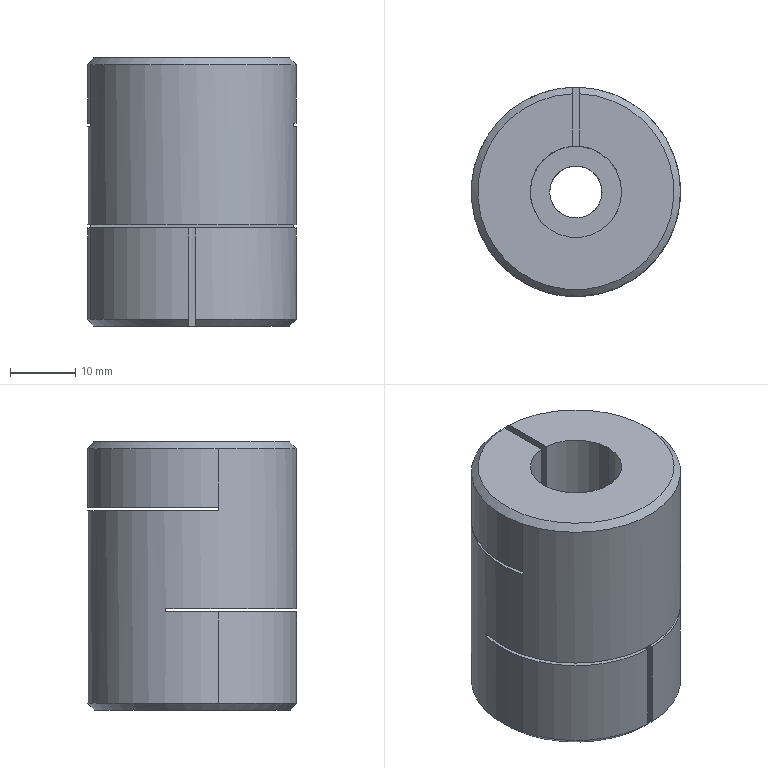Part | NX | 1 solid | 25 faces | box 32 x 32 x 41 mm | volume 27982 mm3 | plane 16 | cylinder 7 | cone 2 | commonest cylinder face diameters 32 x3 8 x2 14 x2
STEP:
#1=CARTESIAN_POINT('',(0.5,-3.969,-5.5));
#2=VERTEX_POINT('',#1);
#3=CARTESIAN_POINT('',(0.,4.,-5.5));
#4=VERTEX_POINT('',#3);
#5=CARTESIAN_POINT('',(0.,0.,-5.5));
#6=DIRECTION('',(0.,0.,-1.));
#7=DIRECTION('',(-1.,0.,0.));
#8=AXIS2_PLACEMENT_3D('',#5,#6,#7);
#9=CIRCLE('',#8,4.);
#10=EDGE_CURVE('',#2,#4,#9,.F.);
#11=ORIENTED_EDGE('',*,*,#10,.F.);
#12=CARTESIAN_POINT('',(0.5,-15.992,-5.5));
#13=VERTEX_POINT('',#12);
#14=CARTESIAN_POINT('',(0.5,-16.,-5.5));
#15=DIRECTION('',(0.,-1.,0.));
#16=VECTOR('',#15,1000.);
#17=LINE('',#14,#16);
#18=EDGE_CURVE('',#2,#13,#17,.T.);
#19=ORIENTED_EDGE('',*,*,#18,.T.);
#20=CARTESIAN_POINT('',(15.492,4.,-5.5));
#21=VERTEX_POINT('',#20);
#22=CARTESIAN_POINT('',(0.,0.,-5.5));
#23=DIRECTION('',(0.,0.,-1.));
#24=DIRECTION('',(-1.,0.,0.));
#25=AXIS2_PLACEMENT_3D('',#22,#23,#24);
#26=CIRCLE('',#25,16.);
#27=EDGE_CURVE('',#21,#13,#26,.T.);
#28=ORIENTED_EDGE('',*,*,#27,.F.);
#29=CARTESIAN_POINT('',(-22.75,4.,-5.5));
#30=DIRECTION('',(1.,0.,0.));
#31=VECTOR('',#30,1000.);
#32=LINE('',#29,#31);
#33=EDGE_CURVE('',#4,#21,#32,.T.);
#34=ORIENTED_EDGE('',*,*,#33,.F.);
#35=EDGE_LOOP('',(#11,#19,#28,#34));
#36=FACE_BOUND('',#35,.T.);
#37=CARTESIAN_POINT('',(-22.75,-16.,-5.5));
#38=DIRECTION('',(0.,0.,-1.));
#39=DIRECTION('',(-1.,0.,0.));
#40=AXIS2_PLACEMENT_3D('',#37,#38,#39);
#41=PLANE('',#40);
#42=ADVANCED_FACE('',(#36),#41,.F.);
#43=CARTESIAN_POINT('',(0.5,6.982,10.5));
#44=VERTEX_POINT('',#43);
#45=CARTESIAN_POINT('',(5.745,-4.,10.5));
#46=VERTEX_POINT('',#45);
#47=CARTESIAN_POINT('',(0.,0.,10.5));
#48=DIRECTION('',(0.,0.,1.));
#49=DIRECTION('',(1.,0.,0.));
#50=AXIS2_PLACEMENT_3D('',#47,#48,#49);
#51=CIRCLE('',#50,7.);
#52=EDGE_CURVE('',#44,#46,#51,.F.);
#53=ORIENTED_EDGE('',*,*,#52,.F.);
#54=CARTESIAN_POINT('',(0.5,15.992,10.5));
#55=VERTEX_POINT('',#54);
#56=CARTESIAN_POINT('',(0.5,16.,10.5));
#57=DIRECTION('',(0.,1.,0.));
#58=VECTOR('',#57,1000.);
#59=LINE('',#56,#58);
#60=EDGE_CURVE('',#44,#55,#59,.T.);
#61=ORIENTED_EDGE('',*,*,#60,.T.);
#62=CARTESIAN_POINT('',(15.492,-4.,10.5));
#63=VERTEX_POINT('',#62);
#64=CARTESIAN_POINT('',(0.,0.,10.5));
#65=DIRECTION('',(0.,0.,1.));
#66=DIRECTION('',(1.,0.,0.));
#67=AXIS2_PLACEMENT_3D('',#64,#65,#66);
#68=CIRCLE('',#67,16.);
#69=EDGE_CURVE('',#63,#55,#68,.T.);
#70=ORIENTED_EDGE('',*,*,#69,.F.);
#71=CARTESIAN_POINT('',(-22.75,-4.,10.5));
#72=DIRECTION('',(1.,0.,0.));
#73=VECTOR('',#72,1000.);
#74=LINE('',#71,#73);
#75=EDGE_CURVE('',#46,#63,#74,.T.);
#76=ORIENTED_EDGE('',*,*,#75,.F.);
#77=EDGE_LOOP('',(#53,#61,#70,#76));
#78=FACE_BOUND('',#77,.T.);
#79=CARTESIAN_POINT('',(-22.75,16.,10.5));
#80=DIRECTION('',(0.,0.,1.));
#81=DIRECTION('',(1.,0.,0.));
#82=AXIS2_PLACEMENT_3D('',#79,#80,#81);
#83=PLANE('',#82);
#84=ADVANCED_FACE('',(#78),#83,.F.);
#85=CARTESIAN_POINT('',(0.5,-3.969,-20.5));
#86=VERTEX_POINT('',#85);
#87=CARTESIAN_POINT('',(-0.5,-3.969,-20.5));
#88=VERTEX_POINT('',#87);
#89=CARTESIAN_POINT('',(0.,0.,-20.5));
#90=DIRECTION('',(0.,0.,1.));
#91=DIRECTION('',(1.,0.,0.));
#92=AXIS2_PLACEMENT_3D('',#89,#90,#91);
#93=CIRCLE('',#92,4.);
#94=EDGE_CURVE('',#86,#88,#93,.T.);
#95=ORIENTED_EDGE('',*,*,#94,.F.);
#96=CARTESIAN_POINT('',(0.5,-3.969,-20.5));
#97=DIRECTION('',(0.,0.,1.));
#98=VECTOR('',#97,1000.);
#99=LINE('',#96,#98);
#100=EDGE_CURVE('',#86,#2,#99,.T.);
#101=ORIENTED_EDGE('',*,*,#100,.T.);
#102=ORIENTED_EDGE('',*,*,#10,.T.);
#103=CARTESIAN_POINT('',(-0.5,-3.969,-5.5));
#104=VERTEX_POINT('',#103);
#105=CARTESIAN_POINT('',(0.,0.,-5.5));
#106=DIRECTION('',(0.,0.,-1.));
#107=DIRECTION('',(-1.,0.,0.));
#108=AXIS2_PLACEMENT_3D('',#105,#106,#107);
#109=CIRCLE('',#108,4.);
#110=EDGE_CURVE('',#4,#104,#109,.F.);
#111=ORIENTED_EDGE('',*,*,#110,.T.);
#112=CARTESIAN_POINT('',(-0.5,-3.969,-20.5));
#113=DIRECTION('',(0.,0.,1.));
#114=VECTOR('',#113,1000.);
#115=LINE('',#112,#114);
#116=EDGE_CURVE('',#104,#88,#115,.F.);
#117=ORIENTED_EDGE('',*,*,#116,.T.);
#118=EDGE_LOOP('',(#95,#101,#102,#111,#117));
#119=FACE_BOUND('',#118,.T.);
#120=CARTESIAN_POINT('',(0.,0.,-20.5));
#121=DIRECTION('',(0.,0.,1.));
#122=DIRECTION('',(1.,0.,0.));
#123=AXIS2_PLACEMENT_3D('',#120,#121,#122);
#124=CYLINDRICAL_SURFACE('',#123,4.);
#125=ADVANCED_FACE('',(#119),#124,.F.);
#126=CARTESIAN_POINT('',(0.,4.,-5.));
#127=VERTEX_POINT('',#126);
#128=CARTESIAN_POINT('',(0.,0.,-5.));
#129=DIRECTION('',(0.,0.,1.));
#130=DIRECTION('',(1.,0.,0.));
#131=AXIS2_PLACEMENT_3D('',#128,#129,#130);
#132=CIRCLE('',#131,4.);
#133=EDGE_CURVE('',#127,#127,#132,.F.);
#134=ORIENTED_EDGE('',*,*,#133,.T.);
#135=EDGE_LOOP('',(#134));
#136=FACE_BOUND('',#135,.T.);
#137=CARTESIAN_POINT('',(4.,0.,0.));
#138=VERTEX_POINT('',#137);
#139=CARTESIAN_POINT('',(0.,0.,0.));
#140=DIRECTION('',(0.,0.,1.));
#141=DIRECTION('',(1.,0.,0.));
#142=AXIS2_PLACEMENT_3D('',#139,#140,#141);
#143=CIRCLE('',#142,4.);
#144=EDGE_CURVE('',#138,#138,#143,.F.);
#145=ORIENTED_EDGE('',*,*,#144,.F.);
#146=EDGE_LOOP('',(#145));
#147=FACE_BOUND('',#146,.T.);
#148=CARTESIAN_POINT('',(0.,0.,-20.5));
#149=DIRECTION('',(0.,0.,1.));
#150=DIRECTION('',(1.,0.,0.));
#151=AXIS2_PLACEMENT_3D('',#148,#149,#150);
#152=CYLINDRICAL_SURFACE('',#151,4.);
#153=ADVANCED_FACE('',(#136,#147),#152,.F.);
#154=CARTESIAN_POINT('',(0.5,15.992,19.5));
#155=VERTEX_POINT('',#154);
#156=CARTESIAN_POINT('',(0.5,15.992,20.5));
#157=DIRECTION('',(0.,0.,-1.));
#158=VECTOR('',#157,1000.);
#159=LINE('',#156,#158);
#160=EDGE_CURVE('',#55,#155,#159,.F.);
#161=ORIENTED_EDGE('',*,*,#160,.T.);
#162=CARTESIAN_POINT('',(-0.5,15.992,19.5));
#163=VERTEX_POINT('',#162);
#164=CARTESIAN_POINT('',(0.,0.,19.5));
#165=DIRECTION('',(0.,0.,1.));
#166=DIRECTION('',(1.,0.,0.));
#167=AXIS2_PLACEMENT_3D('',#164,#165,#166);
#168=CIRCLE('',#167,16.);
#169=EDGE_CURVE('',#155,#163,#168,.F.);
#170=ORIENTED_EDGE('',*,*,#169,.T.);
#171=CARTESIAN_POINT('',(-0.5,15.992,10.5));
#172=VERTEX_POINT('',#171);
#173=CARTESIAN_POINT('',(-0.5,15.992,20.5));
#174=DIRECTION('',(0.,0.,-1.));
#175=VECTOR('',#174,1000.);
#176=LINE('',#173,#175);
#177=EDGE_CURVE('',#163,#172,#176,.T.);
#178=ORIENTED_EDGE('',*,*,#177,.T.);
#179=CARTESIAN_POINT('',(-15.492,-4.,10.5));
#180=VERTEX_POINT('',#179);
#181=CARTESIAN_POINT('',(0.,0.,10.5));
#182=DIRECTION('',(0.,0.,1.));
#183=DIRECTION('',(1.,0.,0.));
#184=AXIS2_PLACEMENT_3D('',#181,#182,#183);
#185=CIRCLE('',#184,16.);
#186=EDGE_CURVE('',#172,#180,#185,.T.);
#187=ORIENTED_EDGE('',*,*,#186,.T.);
#188=CARTESIAN_POINT('',(-15.492,-4.,10.));
#189=VERTEX_POINT('',#188);
#190=CARTESIAN_POINT('',(-15.492,-4.,20.5));
#191=DIRECTION('',(0.,0.,-1.));
#192=VECTOR('',#191,1000.);
#193=LINE('',#190,#192);
#194=EDGE_CURVE('',#180,#189,#193,.T.);
#195=ORIENTED_EDGE('',*,*,#194,.T.);
#196=CARTESIAN_POINT('',(15.492,-4.,10.));
#197=VERTEX_POINT('',#196);
#198=CARTESIAN_POINT('',(0.,0.,10.));
#199=DIRECTION('',(0.,0.,-1.));
#200=DIRECTION('',(0.,1.,0.));
#201=AXIS2_PLACEMENT_3D('',#198,#199,#200);
#202=CIRCLE('',#201,16.);
#203=EDGE_CURVE('',#189,#197,#202,.T.);
#204=ORIENTED_EDGE('',*,*,#203,.T.);
#205=CARTESIAN_POINT('',(15.492,-4.,20.5));
#206=DIRECTION('',(0.,0.,-1.));
#207=VECTOR('',#206,1000.);
#208=LINE('',#205,#207);
#209=EDGE_CURVE('',#197,#63,#208,.F.);
#210=ORIENTED_EDGE('',*,*,#209,.T.);
#211=ORIENTED_EDGE('',*,*,#69,.T.);
#212=EDGE_LOOP('',(#161,#170,#178,#187,#195,#204,#210,#211));
#213=FACE_BOUND('',#212,.T.);
#214=CARTESIAN_POINT('',(0.5,-15.992,-19.5));
#215=VERTEX_POINT('',#214);
#216=CARTESIAN_POINT('',(0.5,-15.992,20.5));
#217=DIRECTION('',(0.,0.,-1.));
#218=VECTOR('',#217,1000.);
#219=LINE('',#216,#218);
#220=EDGE_CURVE('',#13,#215,#219,.T.);
#221=ORIENTED_EDGE('',*,*,#220,.T.);
#222=CARTESIAN_POINT('',(-0.5,-15.992,-19.5));
#223=VERTEX_POINT('',#222);
#224=CARTESIAN_POINT('',(0.,0.,-19.5));
#225=DIRECTION('',(0.,0.,1.));
#226=DIRECTION('',(1.,0.,0.));
#227=AXIS2_PLACEMENT_3D('',#224,#225,#226);
#228=CIRCLE('',#227,16.);
#229=EDGE_CURVE('',#215,#223,#228,.T.);
#230=ORIENTED_EDGE('',*,*,#229,.T.);
#231=CARTESIAN_POINT('',(-0.5,-15.992,-5.5));
#232=VERTEX_POINT('',#231);
#233=CARTESIAN_POINT('',(-0.5,-15.992,20.5));
#234=DIRECTION('',(0.,0.,-1.));
#235=VECTOR('',#234,1000.);
#236=LINE('',#233,#235);
#237=EDGE_CURVE('',#223,#232,#236,.F.);
#238=ORIENTED_EDGE('',*,*,#237,.T.);
#239=CARTESIAN_POINT('',(-15.492,4.,-5.5));
#240=VERTEX_POINT('',#239);
#241=CARTESIAN_POINT('',(0.,0.,-5.5));
#242=DIRECTION('',(0.,0.,-1.));
#243=DIRECTION('',(-1.,0.,0.));
#244=AXIS2_PLACEMENT_3D('',#241,#242,#243);
#245=CIRCLE('',#244,16.);
#246=EDGE_CURVE('',#232,#240,#245,.T.);
#247=ORIENTED_EDGE('',*,*,#246,.T.);
#248=CARTESIAN_POINT('',(-15.492,4.,-5.));
#249=VERTEX_POINT('',#248);
#250=CARTESIAN_POINT('',(-15.492,4.,20.5));
#251=DIRECTION('',(0.,0.,-1.));
#252=VECTOR('',#251,1000.);
#253=LINE('',#250,#252);
#254=EDGE_CURVE('',#240,#249,#253,.F.);
#255=ORIENTED_EDGE('',*,*,#254,.T.);
#256=CARTESIAN_POINT('',(15.492,4.,-5.));
#257=VERTEX_POINT('',#256);
#258=CARTESIAN_POINT('',(0.,0.,-5.));
#259=DIRECTION('',(0.,0.,1.));
#260=DIRECTION('',(1.,0.,0.));
#261=AXIS2_PLACEMENT_3D('',#258,#259,#260);
#262=CIRCLE('',#261,16.);
#263=EDGE_CURVE('',#249,#257,#262,.T.);
#264=ORIENTED_EDGE('',*,*,#263,.T.);
#265=CARTESIAN_POINT('',(15.492,4.,20.5));
#266=DIRECTION('',(0.,0.,-1.));
#267=VECTOR('',#266,1000.);
#268=LINE('',#265,#267);
#269=EDGE_CURVE('',#257,#21,#268,.T.);
#270=ORIENTED_EDGE('',*,*,#269,.T.);
#271=ORIENTED_EDGE('',*,*,#27,.T.);
#272=EDGE_LOOP('',(#221,#230,#238,#247,#255,#264,#270,#271));
#273=FACE_BOUND('',#272,.T.);
#274=CARTESIAN_POINT('',(0.,0.,20.5));
#275=DIRECTION('',(0.,0.,-1.));
#276=DIRECTION('',(-1.,0.,0.));
#277=AXIS2_PLACEMENT_3D('',#274,#275,#276);
#278=CYLINDRICAL_SURFACE('',#277,16.);
#279=ADVANCED_FACE('',(#213,#273),#278,.T.);
#280=CARTESIAN_POINT('',(-0.5,14.992,20.5));
#281=VERTEX_POINT('',#280);
#282=CARTESIAN_POINT('',(-0.5,6.982,20.5));
#283=VERTEX_POINT('',#282);
#284=CARTESIAN_POINT('',(-0.5,20.,20.5));
#285=DIRECTION('',(0.,-1.,0.));
#286=VECTOR('',#285,1000.);
#287=LINE('',#284,#286);
#288=EDGE_CURVE('',#281,#283,#287,.T.);
#289=ORIENTED_EDGE('',*,*,#288,.F.);
#290=CARTESIAN_POINT('',(0.5,14.992,20.5));
#291=VERTEX_POINT('',#290);
#292=CARTESIAN_POINT('',(0.,0.,20.5));
#293=DIRECTION('',(0.,0.,1.));
#294=DIRECTION('',(1.,0.,0.));
#295=AXIS2_PLACEMENT_3D('',#292,#293,#294);
#296=CIRCLE('',#295,15.);
#297=EDGE_CURVE('',#281,#291,#296,.T.);
#298=ORIENTED_EDGE('',*,*,#297,.T.);
#299=CARTESIAN_POINT('',(0.5,6.982,20.5));
#300=VERTEX_POINT('',#299);
#301=CARTESIAN_POINT('',(0.5,20.,20.5));
#302=DIRECTION('',(0.,1.,0.));
#303=VECTOR('',#302,1000.);
#304=LINE('',#301,#303);
#305=EDGE_CURVE('',#300,#291,#304,.T.);
#306=ORIENTED_EDGE('',*,*,#305,.F.);
#307=CARTESIAN_POINT('',(0.,0.,20.5));
#308=DIRECTION('',(0.,0.,1.));
#309=DIRECTION('',(1.,0.,0.));
#310=AXIS2_PLACEMENT_3D('',#307,#308,#309);
#311=CIRCLE('',#310,7.);
#312=EDGE_CURVE('',#283,#300,#311,.T.);
#313=ORIENTED_EDGE('',*,*,#312,.F.);
#314=EDGE_LOOP('',(#289,#298,#306,#313));
#315=FACE_BOUND('',#314,.T.);
#316=CARTESIAN_POINT('',(0.,0.,20.5));
#317=DIRECTION('',(0.,0.,1.));
#318=DIRECTION('',(1.,0.,0.));
#319=AXIS2_PLACEMENT_3D('',#316,#317,#318);
#320=PLANE('',#319);
#321=ADVANCED_FACE('',(#315),#320,.T.);
#322=CARTESIAN_POINT('',(-0.5,-14.992,-20.5));
#323=VERTEX_POINT('',#322);
#324=CARTESIAN_POINT('',(-0.5,0.,-20.5));
#325=DIRECTION('',(0.,1.,0.));
#326=VECTOR('',#325,1000.);
#327=LINE('',#324,#326);
#328=EDGE_CURVE('',#323,#88,#327,.T.);
#329=ORIENTED_EDGE('',*,*,#328,.F.);
#330=CARTESIAN_POINT('',(0.5,-14.992,-20.5));
#331=VERTEX_POINT('',#330);
#332=CARTESIAN_POINT('',(0.,0.,-20.5));
#333=DIRECTION('',(0.,0.,1.));
#334=DIRECTION('',(1.,0.,0.));
#335=AXIS2_PLACEMENT_3D('',#332,#333,#334);
#336=CIRCLE('',#335,15.);
#337=EDGE_CURVE('',#323,#331,#336,.F.);
#338=ORIENTED_EDGE('',*,*,#337,.T.);
#339=CARTESIAN_POINT('',(0.5,0.,-20.5));
#340=DIRECTION('',(0.,-1.,0.));
#341=VECTOR('',#340,1000.);
#342=LINE('',#339,#341);
#343=EDGE_CURVE('',#86,#331,#342,.T.);
#344=ORIENTED_EDGE('',*,*,#343,.F.);
#345=ORIENTED_EDGE('',*,*,#94,.T.);
#346=EDGE_LOOP('',(#329,#338,#344,#345));
#347=FACE_BOUND('',#346,.T.);
#348=CARTESIAN_POINT('',(0.,0.,-20.5));
#349=DIRECTION('',(0.,0.,1.));
#350=DIRECTION('',(1.,0.,0.));
#351=AXIS2_PLACEMENT_3D('',#348,#349,#350);
#352=PLANE('',#351);
#353=ADVANCED_FACE('',(#347),#352,.F.);
#354=CARTESIAN_POINT('',(7.,0.,0.));
#355=VERTEX_POINT('',#354);
#356=CARTESIAN_POINT('',(0.,0.,0.));
#357=DIRECTION('',(0.,0.,1.));
#358=DIRECTION('',(1.,0.,0.));
#359=AXIS2_PLACEMENT_3D('',#356,#357,#358);
#360=CIRCLE('',#359,7.);
#361=EDGE_CURVE('',#355,#355,#360,.T.);
#362=ORIENTED_EDGE('',*,*,#361,.T.);
#363=EDGE_LOOP('',(#362));
#364=FACE_BOUND('',#363,.T.);
#365=ORIENTED_EDGE('',*,*,#144,.T.);
#366=EDGE_LOOP('',(#365));
#367=FACE_BOUND('',#366,.T.);
#368=CARTESIAN_POINT('',(0.,0.,0.));
#369=DIRECTION('',(0.,0.,1.));
#370=DIRECTION('',(1.,0.,0.));
#371=AXIS2_PLACEMENT_3D('',#368,#369,#370);
#372=PLANE('',#371);
#373=ADVANCED_FACE('',(#364,#367),#372,.T.);
#374=ORIENTED_EDGE('',*,*,#312,.T.);
#375=CARTESIAN_POINT('',(0.5,6.982,0.));
#376=DIRECTION('',(0.,0.,1.));
#377=VECTOR('',#376,1000.);
#378=LINE('',#375,#377);
#379=EDGE_CURVE('',#300,#44,#378,.F.);
#380=ORIENTED_EDGE('',*,*,#379,.T.);
#381=ORIENTED_EDGE('',*,*,#52,.T.);
#382=CARTESIAN_POINT('',(5.745,-4.,10.));
#383=VERTEX_POINT('',#382);
#384=CARTESIAN_POINT('',(5.745,-4.,0.));
#385=DIRECTION('',(0.,0.,1.));
#386=VECTOR('',#385,1000.);
#387=LINE('',#384,#386);
#388=EDGE_CURVE('',#46,#383,#387,.F.);
#389=ORIENTED_EDGE('',*,*,#388,.T.);
#390=CARTESIAN_POINT('',(-5.745,-4.,10.));
#391=VERTEX_POINT('',#390);
#392=CARTESIAN_POINT('',(0.,0.,10.));
#393=DIRECTION('',(0.,0.,-1.));
#394=DIRECTION('',(0.,1.,0.));
#395=AXIS2_PLACEMENT_3D('',#392,#393,#394);
#396=CIRCLE('',#395,7.);
#397=EDGE_CURVE('',#383,#391,#396,.F.);
#398=ORIENTED_EDGE('',*,*,#397,.T.);
#399=CARTESIAN_POINT('',(-5.745,-4.,10.5));
#400=VERTEX_POINT('',#399);
#401=CARTESIAN_POINT('',(-5.745,-4.,0.));
#402=DIRECTION('',(0.,0.,1.));
#403=VECTOR('',#402,1000.);
#404=LINE('',#401,#403);
#405=EDGE_CURVE('',#391,#400,#404,.T.);
#406=ORIENTED_EDGE('',*,*,#405,.T.);
#407=CARTESIAN_POINT('',(-0.5,6.982,10.5));
#408=VERTEX_POINT('',#407);
#409=CARTESIAN_POINT('',(0.,0.,10.5));
#410=DIRECTION('',(0.,0.,1.));
#411=DIRECTION('',(1.,0.,0.));
#412=AXIS2_PLACEMENT_3D('',#409,#410,#411);
#413=CIRCLE('',#412,7.);
#414=EDGE_CURVE('',#400,#408,#413,.F.);
#415=ORIENTED_EDGE('',*,*,#414,.T.);
#416=CARTESIAN_POINT('',(-0.5,6.982,0.));
#417=DIRECTION('',(0.,0.,1.));
#418=VECTOR('',#417,1000.);
#419=LINE('',#416,#418);
#420=EDGE_CURVE('',#408,#283,#419,.T.);
#421=ORIENTED_EDGE('',*,*,#420,.T.);
#422=EDGE_LOOP('',(#374,#380,#381,#389,#398,#406,#415,#421));
#423=FACE_BOUND('',#422,.T.);
#424=ORIENTED_EDGE('',*,*,#361,.F.);
#425=EDGE_LOOP('',(#424));
#426=FACE_BOUND('',#425,.T.);
#427=CARTESIAN_POINT('',(0.,0.,0.));
#428=DIRECTION('',(0.,0.,1.));
#429=DIRECTION('',(1.,0.,0.));
#430=AXIS2_PLACEMENT_3D('',#427,#428,#429);
#431=CYLINDRICAL_SURFACE('',#430,7.);
#432=ADVANCED_FACE('',(#423,#426),#431,.F.);
#433=ORIENTED_EDGE('',*,*,#186,.F.);
#434=CARTESIAN_POINT('',(-0.5,16.,10.5));
#435=DIRECTION('',(0.,-1.,0.));
#436=VECTOR('',#435,1000.);
#437=LINE('',#434,#436);
#438=EDGE_CURVE('',#172,#408,#437,.T.);
#439=ORIENTED_EDGE('',*,*,#438,.T.);
#440=ORIENTED_EDGE('',*,*,#414,.F.);
#441=CARTESIAN_POINT('',(-22.75,-4.,10.5));
#442=DIRECTION('',(1.,0.,0.));
#443=VECTOR('',#442,1000.);
#444=LINE('',#441,#443);
#445=EDGE_CURVE('',#180,#400,#444,.T.);
#446=ORIENTED_EDGE('',*,*,#445,.F.);
#447=EDGE_LOOP('',(#433,#439,#440,#446));
#448=FACE_BOUND('',#447,.T.);
#449=CARTESIAN_POINT('',(-22.75,16.,10.5));
#450=DIRECTION('',(0.,0.,1.));
#451=DIRECTION('',(1.,0.,0.));
#452=AXIS2_PLACEMENT_3D('',#449,#450,#451);
#453=PLANE('',#452);
#454=ADVANCED_FACE('',(#448),#453,.F.);
#455=CARTESIAN_POINT('',(-22.75,-4.,10.));
#456=DIRECTION('',(1.,0.,0.));
#457=VECTOR('',#456,1000.);
#458=LINE('',#455,#457);
#459=EDGE_CURVE('',#189,#391,#458,.T.);
#460=ORIENTED_EDGE('',*,*,#459,.T.);
#461=ORIENTED_EDGE('',*,*,#397,.F.);
#462=CARTESIAN_POINT('',(-22.75,-4.,10.));
#463=DIRECTION('',(1.,0.,0.));
#464=VECTOR('',#463,1000.);
#465=LINE('',#462,#464);
#466=EDGE_CURVE('',#383,#197,#465,.T.);
#467=ORIENTED_EDGE('',*,*,#466,.T.);
#468=ORIENTED_EDGE('',*,*,#203,.F.);
#469=EDGE_LOOP('',(#460,#461,#467,#468));
#470=FACE_BOUND('',#469,.T.);
#471=CARTESIAN_POINT('',(-22.75,16.,10.));
#472=DIRECTION('',(0.,0.,-1.));
#473=DIRECTION('',(0.,1.,0.));
#474=AXIS2_PLACEMENT_3D('',#471,#472,#473);
#475=PLANE('',#474);
#476=ADVANCED_FACE('',(#470),#475,.F.);
#477=ORIENTED_EDGE('',*,*,#445,.T.);
#478=ORIENTED_EDGE('',*,*,#405,.F.);
#479=ORIENTED_EDGE('',*,*,#459,.F.);
#480=ORIENTED_EDGE('',*,*,#194,.F.);
#481=EDGE_LOOP('',(#477,#478,#479,#480));
#482=FACE_BOUND('',#481,.T.);
#483=CARTESIAN_POINT('',(-22.75,-4.,10.5));
#484=DIRECTION('',(0.,-1.,0.));
#485=DIRECTION('',(0.,0.,-1.));
#486=AXIS2_PLACEMENT_3D('',#483,#484,#485);
#487=PLANE('',#486);
#488=ADVANCED_FACE('',(#482),#487,.F.);
#489=ORIENTED_EDGE('',*,*,#466,.F.);
#490=ORIENTED_EDGE('',*,*,#388,.F.);
#491=ORIENTED_EDGE('',*,*,#75,.T.);
#492=ORIENTED_EDGE('',*,*,#209,.F.);
#493=EDGE_LOOP('',(#489,#490,#491,#492));
#494=FACE_BOUND('',#493,.T.);
#495=CARTESIAN_POINT('',(-22.75,-4.,10.5));
#496=DIRECTION('',(0.,-1.,0.));
#497=DIRECTION('',(0.,0.,-1.));
#498=AXIS2_PLACEMENT_3D('',#495,#496,#497);
#499=PLANE('',#498);
#500=ADVANCED_FACE('',(#494),#499,.F.);
#501=ORIENTED_EDGE('',*,*,#246,.F.);
#502=CARTESIAN_POINT('',(-0.5,-16.,-5.5));
#503=DIRECTION('',(0.,1.,0.));
#504=VECTOR('',#503,1000.);
#505=LINE('',#502,#504);
#506=EDGE_CURVE('',#232,#104,#505,.T.);
#507=ORIENTED_EDGE('',*,*,#506,.T.);
#508=ORIENTED_EDGE('',*,*,#110,.F.);
#509=CARTESIAN_POINT('',(-22.75,4.,-5.5));
#510=DIRECTION('',(1.,0.,0.));
#511=VECTOR('',#510,1000.);
#512=LINE('',#509,#511);
#513=EDGE_CURVE('',#240,#4,#512,.T.);
#514=ORIENTED_EDGE('',*,*,#513,.F.);
#515=EDGE_LOOP('',(#501,#507,#508,#514));
#516=FACE_BOUND('',#515,.T.);
#517=CARTESIAN_POINT('',(-22.75,-16.,-5.5));
#518=DIRECTION('',(0.,0.,-1.));
#519=DIRECTION('',(-1.,0.,0.));
#520=AXIS2_PLACEMENT_3D('',#517,#518,#519);
#521=PLANE('',#520);
#522=ADVANCED_FACE('',(#516),#521,.F.);
#523=CARTESIAN_POINT('',(-22.75,4.,-5.));
#524=DIRECTION('',(1.,0.,0.));
#525=VECTOR('',#524,1000.);
#526=LINE('',#523,#525);
#527=EDGE_CURVE('',#249,#127,#526,.T.);
#528=ORIENTED_EDGE('',*,*,#527,.T.);
#529=ORIENTED_EDGE('',*,*,#133,.F.);
#530=CARTESIAN_POINT('',(-22.75,4.,-5.));
#531=DIRECTION('',(1.,0.,0.));
#532=VECTOR('',#531,1000.);
#533=LINE('',#530,#532);
#534=EDGE_CURVE('',#127,#257,#533,.T.);
#535=ORIENTED_EDGE('',*,*,#534,.T.);
#536=ORIENTED_EDGE('',*,*,#263,.F.);
#537=EDGE_LOOP('',(#528,#529,#535,#536));
#538=FACE_BOUND('',#537,.T.);
#539=CARTESIAN_POINT('',(-22.75,-16.,-5.));
#540=DIRECTION('',(0.,0.,1.));
#541=DIRECTION('',(1.,0.,0.));
#542=AXIS2_PLACEMENT_3D('',#539,#540,#541);
#543=PLANE('',#542);
#544=ADVANCED_FACE('',(#538),#543,.F.);
#545=ORIENTED_EDGE('',*,*,#527,.F.);
#546=ORIENTED_EDGE('',*,*,#254,.F.);
#547=ORIENTED_EDGE('',*,*,#513,.T.);
#548=ORIENTED_EDGE('',*,*,#33,.T.);
#549=ORIENTED_EDGE('',*,*,#269,.F.);
#550=ORIENTED_EDGE('',*,*,#534,.F.);
#551=EDGE_LOOP('',(#545,#546,#547,#548,#549,#550));
#552=FACE_BOUND('',#551,.T.);
#553=CARTESIAN_POINT('',(-22.75,4.,-5.5));
#554=DIRECTION('',(0.,1.,0.));
#555=DIRECTION('',(0.,0.,1.));
#556=AXIS2_PLACEMENT_3D('',#553,#554,#555);
#557=PLANE('',#556);
#558=ADVANCED_FACE('',(#552),#557,.F.);
#559=ORIENTED_EDGE('',*,*,#177,.F.);
#560=CARTESIAN_POINT('',(-0.5,15.992,19.5));
#561=CARTESIAN_POINT('',(-0.5,15.659,19.833));
#562=CARTESIAN_POINT('',(-0.5,15.325,20.167));
#563=CARTESIAN_POINT('',(-0.5,14.992,20.5));
#564=B_SPLINE_CURVE_WITH_KNOTS('',3,(#560,#561,#562,#563),.UNSPECIFIED.,.F.,.F.,(4,4),(0.,0.001415),.UNSPECIFIED.);
#565=EDGE_CURVE('',#163,#281,#564,.T.);
#566=ORIENTED_EDGE('',*,*,#565,.T.);
#567=ORIENTED_EDGE('',*,*,#288,.T.);
#568=ORIENTED_EDGE('',*,*,#420,.F.);
#569=ORIENTED_EDGE('',*,*,#438,.F.);
#570=EDGE_LOOP('',(#559,#566,#567,#568,#569));
#571=FACE_BOUND('',#570,.T.);
#572=CARTESIAN_POINT('',(-0.5,20.,-10.025));
#573=DIRECTION('',(-1.,0.,0.));
#574=DIRECTION('',(0.,-1.,0.));
#575=AXIS2_PLACEMENT_3D('',#572,#573,#574);
#576=PLANE('',#575);
#577=ADVANCED_FACE('',(#571),#576,.F.);
#578=ORIENTED_EDGE('',*,*,#305,.T.);
#579=CARTESIAN_POINT('',(0.5,14.992,20.5));
#580=CARTESIAN_POINT('',(0.5,15.325,20.167));
#581=CARTESIAN_POINT('',(0.5,15.659,19.833));
#582=CARTESIAN_POINT('',(0.5,15.992,19.5));
#583=B_SPLINE_CURVE_WITH_KNOTS('',3,(#579,#580,#581,#582),.UNSPECIFIED.,.F.,.F.,(4,4),(0.,0.001415),.UNSPECIFIED.);
#584=EDGE_CURVE('',#291,#155,#583,.T.);
#585=ORIENTED_EDGE('',*,*,#584,.T.);
#586=ORIENTED_EDGE('',*,*,#160,.F.);
#587=ORIENTED_EDGE('',*,*,#60,.F.);
#588=ORIENTED_EDGE('',*,*,#379,.F.);
#589=EDGE_LOOP('',(#578,#585,#586,#587,#588));
#590=FACE_BOUND('',#589,.T.);
#591=CARTESIAN_POINT('',(0.5,20.,-10.025));
#592=DIRECTION('',(1.,0.,0.));
#593=DIRECTION('',(0.,1.,0.));
#594=AXIS2_PLACEMENT_3D('',#591,#592,#593);
#595=PLANE('',#594);
#596=ADVANCED_FACE('',(#590),#595,.F.);
#597=ORIENTED_EDGE('',*,*,#237,.F.);
#598=CARTESIAN_POINT('',(-0.5,-15.992,-19.5));
#599=CARTESIAN_POINT('',(-0.5,-15.659,-19.833));
#600=CARTESIAN_POINT('',(-0.5,-15.325,-20.167));
#601=CARTESIAN_POINT('',(-0.5,-14.992,-20.5));
#602=B_SPLINE_CURVE_WITH_KNOTS('',3,(#598,#599,#600,#601),.UNSPECIFIED.,.F.,.F.,(4,4),(0.,0.001415),.UNSPECIFIED.);
#603=EDGE_CURVE('',#223,#323,#602,.T.);
#604=ORIENTED_EDGE('',*,*,#603,.T.);
#605=ORIENTED_EDGE('',*,*,#328,.T.);
#606=ORIENTED_EDGE('',*,*,#116,.F.);
#607=ORIENTED_EDGE('',*,*,#506,.F.);
#608=EDGE_LOOP('',(#597,#604,#605,#606,#607));
#609=FACE_BOUND('',#608,.T.);
#610=CARTESIAN_POINT('',(-0.5,0.,20.02));
#611=DIRECTION('',(-1.,0.,0.));
#612=DIRECTION('',(0.,-1.,0.));
#613=AXIS2_PLACEMENT_3D('',#610,#611,#612);
#614=PLANE('',#613);
#615=ADVANCED_FACE('',(#609),#614,.F.);
#616=ORIENTED_EDGE('',*,*,#343,.T.);
#617=CARTESIAN_POINT('',(0.5,-14.992,-20.5));
#618=CARTESIAN_POINT('',(0.5,-15.325,-20.167));
#619=CARTESIAN_POINT('',(0.5,-15.659,-19.833));
#620=CARTESIAN_POINT('',(0.5,-15.992,-19.5));
#621=B_SPLINE_CURVE_WITH_KNOTS('',3,(#617,#618,#619,#620),.UNSPECIFIED.,.F.,.F.,(4,4),(0.,0.001415),.UNSPECIFIED.);
#622=EDGE_CURVE('',#331,#215,#621,.T.);
#623=ORIENTED_EDGE('',*,*,#622,.T.);
#624=ORIENTED_EDGE('',*,*,#220,.F.);
#625=ORIENTED_EDGE('',*,*,#18,.F.);
#626=ORIENTED_EDGE('',*,*,#100,.F.);
#627=EDGE_LOOP('',(#616,#623,#624,#625,#626));
#628=FACE_BOUND('',#627,.T.);
#629=CARTESIAN_POINT('',(0.5,0.,20.02));
#630=DIRECTION('',(1.,0.,0.));
#631=DIRECTION('',(0.,1.,0.));
#632=AXIS2_PLACEMENT_3D('',#629,#630,#631);
#633=PLANE('',#632);
#634=ADVANCED_FACE('',(#628),#633,.F.);
#635=ORIENTED_EDGE('',*,*,#565,.F.);
#636=ORIENTED_EDGE('',*,*,#169,.F.);
#637=ORIENTED_EDGE('',*,*,#584,.F.);
#638=ORIENTED_EDGE('',*,*,#297,.F.);
#639=EDGE_LOOP('',(#635,#636,#637,#638));
#640=FACE_BOUND('',#639,.T.);
#641=CARTESIAN_POINT('',(0.,0.,20.5));
#642=DIRECTION('',(0.,0.,-1.));
#643=DIRECTION('',(-1.,0.,0.));
#644=AXIS2_PLACEMENT_3D('',#641,#642,#643);
#645=CONICAL_SURFACE('',#644,15.,0.7854);
#646=ADVANCED_FACE('',(#640),#645,.T.);
#647=ORIENTED_EDGE('',*,*,#622,.F.);
#648=ORIENTED_EDGE('',*,*,#337,.F.);
#649=ORIENTED_EDGE('',*,*,#603,.F.);
#650=ORIENTED_EDGE('',*,*,#229,.F.);
#651=EDGE_LOOP('',(#647,#648,#649,#650));
#652=FACE_BOUND('',#651,.T.);
#653=CARTESIAN_POINT('',(0.,0.,-19.5));
#654=DIRECTION('',(0.,0.,1.));
#655=DIRECTION('',(1.,0.,0.));
#656=AXIS2_PLACEMENT_3D('',#653,#654,#655);
#657=CONICAL_SURFACE('',#656,16.,0.7854);
#658=ADVANCED_FACE('',(#652),#657,.T.);
#659=CLOSED_SHELL('',(#42,#84,#125,#153,#279,#321,#353,#373,#432,#454,#476,#488,#500,#522,#544,#558,#577,#596,#615,#634,#646,#658));
#660=MANIFOLD_SOLID_BREP('',#659);
#661=(LENGTH_UNIT()NAMED_UNIT(*)SI_UNIT(.MILLI.,.METRE.));
#662=UNCERTAINTY_MEASURE_WITH_UNIT(LENGTH_MEASURE(0.0508),#661,'','');
#663=(NAMED_UNIT(*)PLANE_ANGLE_UNIT()SI_UNIT($,.RADIAN.));
#664=(NAMED_UNIT(*)SI_UNIT($,.STERADIAN.)SOLID_ANGLE_UNIT());
#665=(GEOMETRIC_REPRESENTATION_CONTEXT(3)GLOBAL_UNCERTAINTY_ASSIGNED_CONTEXT((#662))GLOBAL_UNIT_ASSIGNED_CONTEXT((#661,#663,#664))REPRESENTATION_CONTEXT('',''));
#666=ADVANCED_BREP_SHAPE_REPRESENTATION('',(#660),#665);